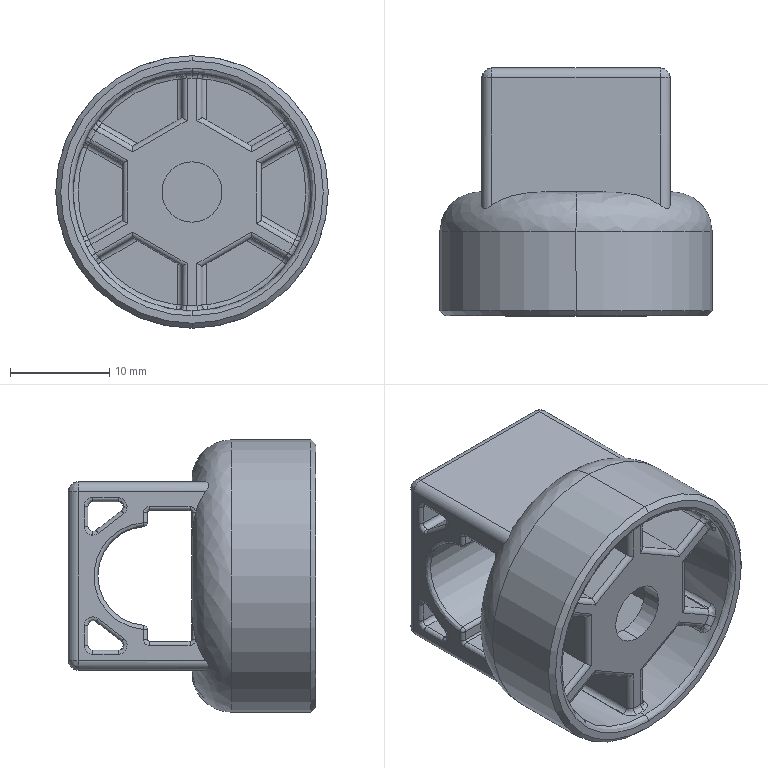Part | SolidWorks | 1 solid | 231 faces | box 27.5 x 25 x 27.5 mm | volume 6208 mm3 | cylinder 98 | spline 73 | plane 58 | cone 2 | commonest cylinder face diameters 1 x53 0.8 x26 2 x8 0.4 x4 6.1 x2 24 x2